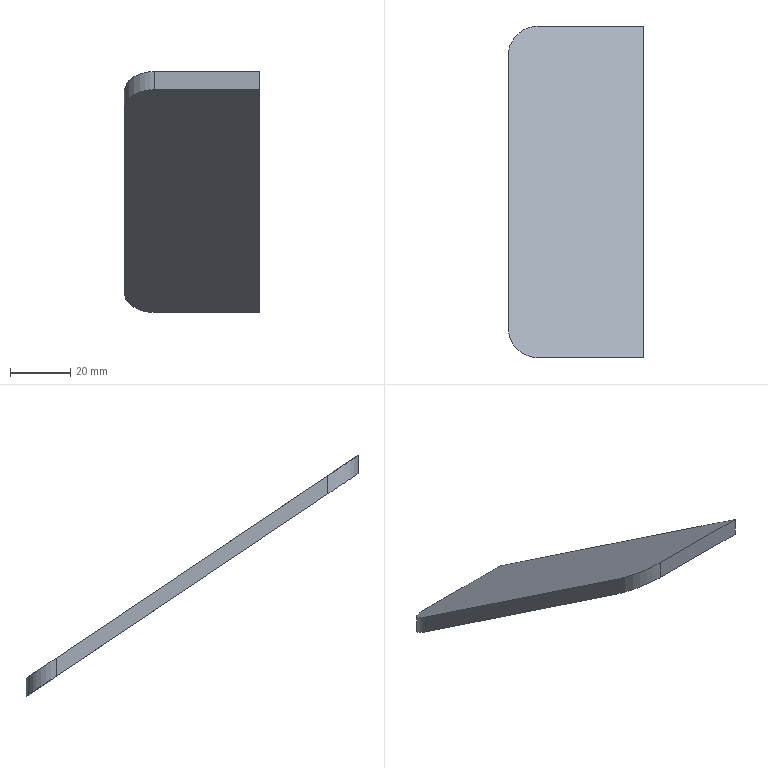Part | SolidWorks | features Extrusion 1, ICE 1 | 1 solid | 8 faces | box 45 x 110 x 79.839 mm | volume 29548 mm3 | plane 6 | cylinder 2 | commonest cylinder face diameters 20 x2
STEP:
#1=CARTESIAN_POINT('',(-679.821,67.7,12.204));
#2=VERTEX_POINT('',#1);
#3=CARTESIAN_POINT('',(-679.821,67.7,6.182));
#4=VERTEX_POINT('',#3);
#5=CARTESIAN_POINT('',(-679.821,67.7,100.));
#6=DIRECTION('',(0.,0.,-1.));
#7=VECTOR('',#6,1000.);
#8=LINE('',#5,#7);
#9=EDGE_CURVE('',#2,#4,#8,.T.);
#10=ORIENTED_EDGE('',*,*,#9,.F.);
#11=CARTESIAN_POINT('',(-679.821,-42.3,86.021));
#12=VERTEX_POINT('',#11);
#13=CARTESIAN_POINT('',(-679.821,26.668,39.739));
#14=DIRECTION('',(0.,-0.8304,0.5572));
#15=VECTOR('',#14,1000.);
#16=LINE('',#13,#15);
#17=EDGE_CURVE('',#2,#12,#16,.T.);
#18=ORIENTED_EDGE('',*,*,#17,.T.);
#19=CARTESIAN_POINT('',(-679.821,-42.3,80.));
#20=VERTEX_POINT('',#19);
#21=CARTESIAN_POINT('',(-679.821,-42.3,100.));
#22=DIRECTION('',(0.,0.,-1.));
#23=VECTOR('',#22,1000.);
#24=LINE('',#21,#23);
#25=EDGE_CURVE('',#12,#20,#24,.T.);
#26=ORIENTED_EDGE('',*,*,#25,.T.);
#27=CARTESIAN_POINT('',(-679.821,23.882,35.588));
#28=DIRECTION('',(0.,-0.8304,0.5572));
#29=VECTOR('',#28,1000.);
#30=LINE('',#27,#29);
#31=EDGE_CURVE('',#4,#20,#30,.T.);
#32=ORIENTED_EDGE('',*,*,#31,.F.);
#33=EDGE_LOOP('',(#10,#18,#26,#32));
#34=FACE_OUTER_BOUND('',#33,.T.);
#35=CARTESIAN_POINT('',(-679.821,67.7,100.));
#36=DIRECTION('',(1.,0.,0.));
#37=DIRECTION('',(0.,1.,0.));
#38=AXIS2_PLACEMENT_3D('',#35,#36,#37);
#39=PLANE('',#38);
#40=ADVANCED_FACE('',(#34),#39,.T.);
#41=CARTESIAN_POINT('',(-714.821,67.7,12.204));
#42=VERTEX_POINT('',#41);
#43=CARTESIAN_POINT('',(-779.821,67.7,12.204));
#44=DIRECTION('',(1.,0.,0.));
#45=VECTOR('',#44,1000.);
#46=LINE('',#43,#45);
#47=EDGE_CURVE('',#42,#2,#46,.T.);
#48=ORIENTED_EDGE('',*,*,#47,.T.);
#49=ORIENTED_EDGE('',*,*,#9,.T.);
#50=CARTESIAN_POINT('',(-714.821,67.7,6.182));
#51=VERTEX_POINT('',#50);
#52=CARTESIAN_POINT('',(-779.821,67.7,6.182));
#53=DIRECTION('',(1.,0.,0.));
#54=VECTOR('',#53,1000.);
#55=LINE('',#52,#54);
#56=EDGE_CURVE('',#51,#4,#55,.T.);
#57=ORIENTED_EDGE('',*,*,#56,.F.);
#58=CARTESIAN_POINT('',(-714.821,67.7,100.));
#59=DIRECTION('',(0.,0.,-1.));
#60=VECTOR('',#59,1000.);
#61=LINE('',#58,#60);
#62=EDGE_CURVE('',#42,#51,#61,.T.);
#63=ORIENTED_EDGE('',*,*,#62,.F.);
#64=EDGE_LOOP('',(#48,#49,#57,#63));
#65=FACE_OUTER_BOUND('',#64,.T.);
#66=CARTESIAN_POINT('',(-679.821,67.7,100.));
#67=DIRECTION('',(0.,-1.,0.));
#68=DIRECTION('',(1.,0.,0.));
#69=AXIS2_PLACEMENT_3D('',#66,#67,#68);
#70=PLANE('',#69);
#71=ADVANCED_FACE('',(#65),#70,.F.);
#72=CARTESIAN_POINT('',(-724.821,57.7,18.915));
#73=VERTEX_POINT('',#72);
#74=CARTESIAN_POINT('',(-714.821,67.7,12.204));
#75=CARTESIAN_POINT('',(-720.679,67.7,12.204));
#76=CARTESIAN_POINT('',(-724.821,63.558,14.984));
#77=CARTESIAN_POINT('',(-724.821,57.7,18.915));
#78=(BOUNDED_CURVE()B_SPLINE_CURVE(3,(#74,#75,#76,#77),.UNSPECIFIED.,.F.,.F.)B_SPLINE_CURVE_WITH_KNOTS((4,4),(0.,1.571),.UNSPECIFIED.)CURVE()GEOMETRIC_REPRESENTATION_ITEM()RATIONAL_B_SPLINE_CURVE((1.,0.8047,0.8047,1.))REPRESENTATION_ITEM(''));
#79=EDGE_CURVE('',#42,#73,#78,.T.);
#80=ORIENTED_EDGE('',*,*,#79,.F.);
#81=ORIENTED_EDGE('',*,*,#62,.T.);
#82=CARTESIAN_POINT('',(-724.821,57.7,12.893));
#83=VERTEX_POINT('',#82);
#84=CARTESIAN_POINT('',(-714.821,67.7,6.182));
#85=CARTESIAN_POINT('',(-720.679,67.7,6.182));
#86=CARTESIAN_POINT('',(-724.821,63.558,8.962));
#87=CARTESIAN_POINT('',(-724.821,57.7,12.893));
#88=(BOUNDED_CURVE()B_SPLINE_CURVE(3,(#84,#85,#86,#87),.UNSPECIFIED.,.F.,.F.)B_SPLINE_CURVE_WITH_KNOTS((4,4),(0.,1.571),.UNSPECIFIED.)CURVE()GEOMETRIC_REPRESENTATION_ITEM()RATIONAL_B_SPLINE_CURVE((1.,0.8047,0.8047,1.))REPRESENTATION_ITEM(''));
#89=EDGE_CURVE('',#51,#83,#88,.T.);
#90=ORIENTED_EDGE('',*,*,#89,.T.);
#91=CARTESIAN_POINT('',(-724.821,57.7,100.));
#92=DIRECTION('',(0.,0.,-1.));
#93=VECTOR('',#92,1000.);
#94=LINE('',#91,#93);
#95=EDGE_CURVE('',#73,#83,#94,.T.);
#96=ORIENTED_EDGE('',*,*,#95,.F.);
#97=EDGE_LOOP('',(#80,#81,#90,#96));
#98=FACE_OUTER_BOUND('',#97,.T.);
#99=CARTESIAN_POINT('',(-714.821,57.7,100.));
#100=DIRECTION('',(0.,0.,-1.));
#101=DIRECTION('',(-1.,0.,0.));
#102=AXIS2_PLACEMENT_3D('',#99,#100,#101);
#103=CYLINDRICAL_SURFACE('',#102,10.);
#104=ADVANCED_FACE('',(#98),#103,.T.);
#105=CARTESIAN_POINT('',(-724.821,-32.3,79.311));
#106=VERTEX_POINT('',#105);
#107=CARTESIAN_POINT('',(-724.821,-32.3,73.289));
#108=VERTEX_POINT('',#107);
#109=CARTESIAN_POINT('',(-724.821,-32.3,100.));
#110=DIRECTION('',(0.,0.,-1.));
#111=VECTOR('',#110,1000.);
#112=LINE('',#109,#111);
#113=EDGE_CURVE('',#106,#108,#112,.T.);
#114=ORIENTED_EDGE('',*,*,#113,.F.);
#115=CARTESIAN_POINT('',(-724.821,-41.873,85.735));
#116=DIRECTION('',(0.,0.8304,-0.5572));
#117=VECTOR('',#116,1000.);
#118=LINE('',#115,#117);
#119=EDGE_CURVE('',#106,#73,#118,.T.);
#120=ORIENTED_EDGE('',*,*,#119,.T.);
#121=ORIENTED_EDGE('',*,*,#95,.T.);
#122=CARTESIAN_POINT('',(-724.821,-44.659,81.583));
#123=DIRECTION('',(0.,0.8304,-0.5572));
#124=VECTOR('',#123,1000.);
#125=LINE('',#122,#124);
#126=EDGE_CURVE('',#108,#83,#125,.T.);
#127=ORIENTED_EDGE('',*,*,#126,.F.);
#128=EDGE_LOOP('',(#114,#120,#121,#127));
#129=FACE_OUTER_BOUND('',#128,.T.);
#130=CARTESIAN_POINT('',(-724.821,-32.3,100.));
#131=DIRECTION('',(-1.,0.,0.));
#132=DIRECTION('',(0.,0.,1.));
#133=AXIS2_PLACEMENT_3D('',#130,#131,#132);
#134=PLANE('',#133);
#135=ADVANCED_FACE('',(#129),#134,.T.);
#136=CARTESIAN_POINT('',(-714.821,-42.3,86.021));
#137=VERTEX_POINT('',#136);
#138=CARTESIAN_POINT('',(-724.821,-32.3,79.311));
#139=CARTESIAN_POINT('',(-724.821,-38.158,83.242));
#140=CARTESIAN_POINT('',(-720.679,-42.3,86.021));
#141=CARTESIAN_POINT('',(-714.821,-42.3,86.021));
#142=(BOUNDED_CURVE()B_SPLINE_CURVE(3,(#138,#139,#140,#141),.UNSPECIFIED.,.F.,.F.)B_SPLINE_CURVE_WITH_KNOTS((4,4),(1.571,3.142),.UNSPECIFIED.)CURVE()GEOMETRIC_REPRESENTATION_ITEM()RATIONAL_B_SPLINE_CURVE((1.,0.8047,0.8047,1.))REPRESENTATION_ITEM(''));
#143=EDGE_CURVE('',#106,#137,#142,.T.);
#144=ORIENTED_EDGE('',*,*,#143,.F.);
#145=ORIENTED_EDGE('',*,*,#113,.T.);
#146=CARTESIAN_POINT('',(-714.821,-42.3,80.));
#147=VERTEX_POINT('',#146);
#148=CARTESIAN_POINT('',(-724.821,-32.3,73.289));
#149=CARTESIAN_POINT('',(-724.821,-38.158,77.22));
#150=CARTESIAN_POINT('',(-720.679,-42.3,80.));
#151=CARTESIAN_POINT('',(-714.821,-42.3,80.));
#152=(BOUNDED_CURVE()B_SPLINE_CURVE(3,(#148,#149,#150,#151),.UNSPECIFIED.,.F.,.F.)B_SPLINE_CURVE_WITH_KNOTS((4,4),(1.571,3.142),.UNSPECIFIED.)CURVE()GEOMETRIC_REPRESENTATION_ITEM()RATIONAL_B_SPLINE_CURVE((1.,0.8047,0.8047,1.))REPRESENTATION_ITEM(''));
#153=EDGE_CURVE('',#108,#147,#152,.T.);
#154=ORIENTED_EDGE('',*,*,#153,.T.);
#155=CARTESIAN_POINT('',(-714.821,-42.3,100.));
#156=DIRECTION('',(0.,0.,-1.));
#157=VECTOR('',#156,1000.);
#158=LINE('',#155,#157);
#159=EDGE_CURVE('',#137,#147,#158,.T.);
#160=ORIENTED_EDGE('',*,*,#159,.F.);
#161=EDGE_LOOP('',(#144,#145,#154,#160));
#162=FACE_OUTER_BOUND('',#161,.T.);
#163=CARTESIAN_POINT('',(-714.821,-32.3,100.));
#164=DIRECTION('',(0.,0.,-1.));
#165=DIRECTION('',(-1.,0.,0.));
#166=AXIS2_PLACEMENT_3D('',#163,#164,#165);
#167=CYLINDRICAL_SURFACE('',#166,10.);
#168=ADVANCED_FACE('',(#162),#167,.T.);
#169=ORIENTED_EDGE('',*,*,#25,.F.);
#170=CARTESIAN_POINT('',(-679.821,-42.3,86.021));
#171=DIRECTION('',(-1.,0.,0.));
#172=VECTOR('',#171,1000.);
#173=LINE('',#170,#172);
#174=EDGE_CURVE('',#12,#137,#173,.T.);
#175=ORIENTED_EDGE('',*,*,#174,.T.);
#176=ORIENTED_EDGE('',*,*,#159,.T.);
#177=CARTESIAN_POINT('',(-679.821,-42.3,80.));
#178=DIRECTION('',(-1.,0.,0.));
#179=VECTOR('',#178,1000.);
#180=LINE('',#177,#179);
#181=EDGE_CURVE('',#20,#147,#180,.T.);
#182=ORIENTED_EDGE('',*,*,#181,.F.);
#183=EDGE_LOOP('',(#169,#175,#176,#182));
#184=FACE_OUTER_BOUND('',#183,.T.);
#185=CARTESIAN_POINT('',(-679.821,-42.3,100.));
#186=DIRECTION('',(0.,-1.,0.));
#187=DIRECTION('',(1.,0.,0.));
#188=AXIS2_PLACEMENT_3D('',#185,#186,#187);
#189=PLANE('',#188);
#190=ADVANCED_FACE('',(#184),#189,.T.);
#191=ORIENTED_EDGE('',*,*,#56,.T.);
#192=ORIENTED_EDGE('',*,*,#31,.T.);
#193=ORIENTED_EDGE('',*,*,#181,.T.);
#194=ORIENTED_EDGE('',*,*,#153,.F.);
#195=ORIENTED_EDGE('',*,*,#126,.T.);
#196=ORIENTED_EDGE('',*,*,#89,.F.);
#197=EDGE_LOOP('',(#191,#192,#193,#194,#195,#196));
#198=FACE_OUTER_BOUND('',#197,.T.);
#199=CARTESIAN_POINT('',(-779.821,23.882,35.588));
#200=DIRECTION('',(0.,0.5572,0.8304));
#201=DIRECTION('',(0.,-0.8304,0.5572));
#202=AXIS2_PLACEMENT_3D('',#199,#200,#201);
#203=PLANE('',#202);
#204=ADVANCED_FACE('',(#198),#203,.F.);
#205=ORIENTED_EDGE('',*,*,#79,.T.);
#206=ORIENTED_EDGE('',*,*,#119,.F.);
#207=ORIENTED_EDGE('',*,*,#143,.T.);
#208=ORIENTED_EDGE('',*,*,#174,.F.);
#209=ORIENTED_EDGE('',*,*,#17,.F.);
#210=ORIENTED_EDGE('',*,*,#47,.F.);
#211=EDGE_LOOP('',(#205,#206,#207,#208,#209,#210));
#212=FACE_OUTER_BOUND('',#211,.T.);
#213=CARTESIAN_POINT('',(-779.821,26.668,39.739));
#214=DIRECTION('',(0.,0.5572,0.8304));
#215=DIRECTION('',(0.,-0.8304,0.5572));
#216=AXIS2_PLACEMENT_3D('',#213,#214,#215);
#217=PLANE('',#216);
#218=ADVANCED_FACE('',(#212),#217,.T.);
#219=CLOSED_SHELL('',(#40,#71,#104,#135,#168,#190,#204,#218));
#220=MANIFOLD_SOLID_BREP('',#219);
#221=CARTESIAN_POINT('',(0.,0.,0.));
#222=DIRECTION('',(0.,0.,1.));
#223=DIRECTION('',(1.,0.,0.));
#224=AXIS2_PLACEMENT_3D('',#221,#222,#223);
#225=(LENGTH_UNIT()NAMED_UNIT(*)SI_UNIT(.MILLI.,.METRE.));
#226=UNCERTAINTY_MEASURE_WITH_UNIT(LENGTH_MEASURE(0.00001),#225,'','');
#227=(NAMED_UNIT(*)PLANE_ANGLE_UNIT()SI_UNIT($,.RADIAN.));
#228=(NAMED_UNIT(*)SI_UNIT($,.STERADIAN.)SOLID_ANGLE_UNIT());
#229=(GEOMETRIC_REPRESENTATION_CONTEXT(3)GLOBAL_UNCERTAINTY_ASSIGNED_CONTEXT((#226))GLOBAL_UNIT_ASSIGNED_CONTEXT((#225,#227,#228))REPRESENTATION_CONTEXT('',''));
#230=ADVANCED_BREP_SHAPE_REPRESENTATION('',(#220,#224),#229);